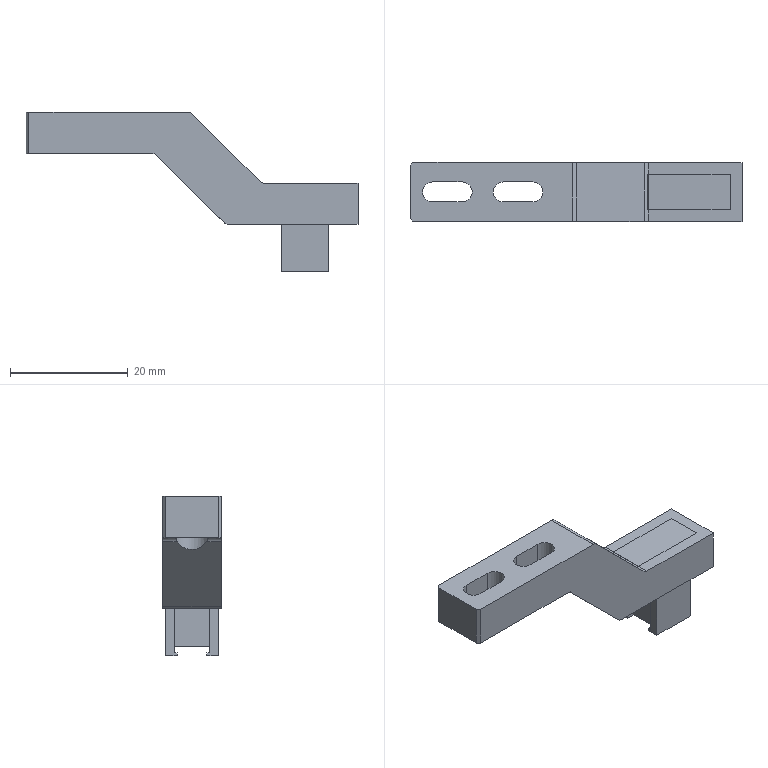NC program | NX | posted with a generic post | part box 56.3 x 10 x 27 mm
Lines 2463 to 3920 of 3920:
(ZLEVEL_PROFILE_COPY_1_COPY , TOOL : D4R0.2)
N4900 T05 M6
N4902 G54
N4904 G17 G0 G90 X3.577 Y-6.289 S9500 M3
N4906 G43 Z30. H5
N4908 Z-6.511
N4910 G94 G1 Z-8.011 F800.
N4912 X4.098 Y-5.88
N4914 G3 X4.247 Y-5.509 R0.4
N4916 G1 X4.175 Y-5. F2000.
N4918 Y5.
N4920 X4.242 Y5.476
N4922 X4.254 Y5.53
N4924 X4.194 Y5.54 Z-8.023
N4926 X4.108 Y5.
N4928 Y-5.
N4930 X4.186 Y-5.505
N4932 X4.154 Y-5.504 Z-8.029
N4934 X4.079 Y-5.
N4936 Y5.
N4938 G2 X4.166 Y5.547 R2.006
N4940 G1 X4.13 Y5.551 Z-8.038
N4942 X4.095 Y5.555 Z-8.047
N4944 X4.008 Y5.
N4946 Y-5.
N4948 X4.08 Y-5.501
N4950 X4.037 Y-5.503 Z-8.061
N4952 X3.994 Y-5.505 Z-8.074
N4954 X3.924 Y-5.
N4956 Y5.
N4958 X3.988 Y5.476
N4960 X4.009 Y5.55
N4962 X3.923 Y5.537 Z-8.109
N4964 X3.84 Y5.
N4966 Y-5.
N4968 X3.913 Y-5.503
N4970 X3.865 Y-5.502 Z-8.13
N4972 X3.825 Y-5.5 Z-8.15
N4974 X3.758 Y-5.
N4976 Y5.
N4978 X3.83 Y5.518
N4980 X3.791 Y5.517 Z-8.175
N4982 X3.749 Y5.516 Z-8.199
N4984 X3.678 Y5.
N4986 Y-5.
N4988 X3.747 Y-5.502
N4990 X3.708 Z-8.227
N4992 X3.667 Z-8.255
N4994 X3.6 Y-5.
N4996 Y5.
N4998 X3.668 Y5.511
N5000 X3.631 Y5.507 Z-8.286
N5002 X3.588 Y5.503 Z-8.317
N5004 G3 X3.527 Y5. R5.351
N5006 G1 Y-5.
N5008 G3 X3.589 Y-5.501 R2.547
N5010 G1 X3.549 Y-5.5 Z-8.35
N5012 X3.513 Z-8.384
N5014 G2 X3.458 Y-5. R31.618
N5016 G1 Y5.
N5018 X3.511 Y5.5
N5020 X3.47 Z-8.418
N5022 X3.439 Z-8.452
N5024 X3.39 Y5.
N5026 Y-5.
N5028 G3 X3.441 Y-5.5 R21.316
N5030 G1 X3.404 Z-8.487
N5032 X3.369 Z-8.521
N5034 G2 X3.32 Y-5. R27.436
N5036 G1 Y5.
N5038 X3.366 Y5.5
N5040 X3.326 Z-8.556
N5042 X3.292 Z-8.591
N5044 X3.25 Y5.
N5046 Y-5.
N5048 G3 X3.295 Y-5.5 R22.467
N5050 G1 X3.258 Z-8.626
N5052 X3.222 Z-8.662
N5054 G2 X3.179 Y-5. R2.843
N5056 G1 Y5.
N5058 X3.218 Y5.5
N5060 X3.18 Z-8.697
N5062 X3.145 Z-8.732
N5064 X3.108 Y5.
N5066 Y-5.
N5068 G3 X3.148 Y-5.5 R26.717
N5070 G1 X3.111 Z-8.767
N5072 X3.075 Z-8.803
N5074 X3.037 Y-5.
N5076 Y5.
N5078 X3.072 Y5.5
N5080 X3.034 Z-8.838
N5082 X2.999 Z-8.873
N5084 X2.966 Y5.
N5086 Y-5.
N5088 X3.001 Y-5.5
N5090 X2.964 Z-8.908
N5092 X2.928 Z-8.944
N5094 X2.895 Y-5.
N5096 Y5.
N5098 X2.926 Y5.5
N5100 X2.888 Z-8.979
N5102 X2.853 Z-9.014
N5104 X2.825 Y5.
N5106 Y-5.
N5108 X2.854 Y-5.5
N5110 X2.817 Z-9.05
N5112 X2.781 Z-9.085
N5114 X2.754 Y-5.
N5116 Y5.
N5118 X2.779 Y5.5
N5120 X2.741 Z-9.12
N5122 X2.706 Z-9.155
N5124 X2.683 Y5.
N5126 Y-5.
N5128 X2.707 Y-5.5
N5130 X2.67 Z-9.191
N5132 X2.635 Z-9.226
N5134 X2.612 Y-5.
N5136 Y5.
N5138 X2.633 Y5.5
N5140 X2.595 Z-9.261
N5142 X2.56 Z-9.296
N5144 X2.541 Y5.
N5146 Y-5.
N5148 X2.561 Y-5.5
N5150 X2.524 Z-9.332
N5152 X2.488 Z-9.367
N5154 X2.47 Y-5.
N5156 Y5.
N5158 X2.487 Y5.5
N5160 X2.449 Z-9.402
N5162 X2.414 Z-9.437
N5164 X2.399 Y5.
N5166 Y-5.
N5168 X2.415 Y-5.5
N5170 X2.378 Z-9.473
N5172 X2.342 Z-9.508
N5174 X2.328 Y-5.
N5176 Y5.
N5178 X2.34 Y5.5
N5180 X2.302 Z-9.543
N5182 X2.267 Z-9.578
N5184 X2.257 Y5.
N5186 Y-5.
N5188 X2.269 Y-5.5
N5190 X2.232 Z-9.614
N5192 X2.196 Z-9.649
N5194 X2.195 Y-5.476
N5196 X2.186 Y-5.
N5198 Y5.
N5200 X2.194 Y5.5
N5202 X2.156 Z-9.684
N5204 X2.122 Z-9.719
N5206 X2.115 Y5.
N5208 Y-5.
N5210 X2.124 Y-5.5
N5212 X2.087 Z-9.755
N5214 X2.053 Z-9.79
N5216 X2.045 Y-5.
N5218 Y5.
N5220 X2.05 Y5.5
N5222 X2.012 Z-9.825
N5224 X1.979 Z-9.86
N5226 X1.974 Y5.
N5228 Y-5.
N5230 X1.981 Y-5.5
N5232 X1.944 Z-9.896
N5234 X1.91 Z-9.931
N5236 X1.903 Y-5.
N5238 Y5.
N5240 X1.907 Y5.5
N5242 X1.87 Z-9.966
N5244 X1.836 Z-10.001
N5246 X1.832 Y5.
N5248 Y-5.
N5250 X1.838 Y-5.5
N5252 X1.802 Z-10.037
N5254 X1.767 Z-10.072
N5256 X1.761 Y-5.
N5258 Y5.
N5260 X1.765 Y5.5
N5262 X1.728 Z-10.107
N5264 X1.694 Z-10.142
N5266 X1.69 Y5.
N5268 Y-5.
N5270 X1.696 Y-5.5
N5272 X1.659 Z-10.178
N5274 X1.625 Z-10.213
N5276 X1.619 Y-5.
N5278 Y5.
N5280 X1.623 Y5.5
N5282 X1.586 Z-10.248
N5284 X1.552 Z-10.283
N5286 X1.548 Y5.
N5288 Y-5.
N5290 X1.553 Y-5.5
N5292 X1.517 Z-10.319
N5294 X1.482 Z-10.354
N5296 X1.477 Y-5.
N5298 Y5.
N5300 X1.481 Y5.5
N5302 X1.444 Z-10.389
N5304 X1.41 Z-10.424
N5306 X1.406 Y5.
N5308 Y-5.
N5310 X1.409 Y-5.476
N5312 X1.411 Y-5.5
N5314 X1.374 Z-10.46
N5316 X1.34 Z-10.495
N5318 X1.338 Y-5.476
N5320 X1.335 Y-5.
N5322 Y5.
N5324 X1.337 Y5.476
N5326 X1.339 Y5.5
N5328 X1.302 Z-10.53
N5330 X1.268 Z-10.565
N5332 X1.266 Y5.476
N5334 X1.265 Y5.
N5336 Y-5.
N5338 X1.267 Y-5.476
N5340 X1.268 Y-5.5
N5342 X1.232 Z-10.601
N5344 X1.197 Z-10.636
N5346 X1.196 Y-5.476
N5348 X1.194 Y-5.
N5350 Y5.
N5352 X1.195 Y5.476
N5354 X1.196 Y5.5
N5356 X1.159 Z-10.671
N5358 X1.125 Z-10.707
N5360 X1.124 Y5.476
N5362 X1.123 Y5.
N5364 Y-5.
N5366 X1.124 Y-5.476
N5368 X1.126 Y-5.5
N5370 X1.089 Z-10.742
N5372 X1.055 Z-10.777
N5374 X1.053 Y-5.476
N5376 X1.052 Y-5.
N5378 Y5.
N5380 X1.053 Y5.476
N5382 X1.054 Y5.5
N5384 X1.017 Z-10.812
N5386 X0.983 Z-10.848
N5388 X0.982 Y5.476
N5390 X0.981 Y5.
N5392 Y-5.
N5394 X0.982 Y-5.476
N5396 X0.984 Y-5.5
N5398 X0.947 Z-10.883
N5400 X0.912 Z-10.918
N5402 X0.911 Y-5.476
N5404 X0.91 Y-5.
N5406 Y5.
N5408 X0.911 Y5.476
N5410 X0.912 Y5.5
N5412 X0.875 Z-10.953
N5414 X0.841 Z-10.989
N5416 X0.84 Y5.476
N5418 X0.839 Y5.
N5420 Y-5.
N5422 X0.84 Y-5.476
N5424 X0.841 Y-5.5
N5426 X0.804 Z-11.024
N5428 X0.77 Z-11.059
N5430 X0.769 Y-5.476
N5432 X0.768 Y-5.
N5434 Y5.
N5436 X0.769 Y5.476
N5438 X0.77 Y5.5
N5440 X0.733 Z-11.094
N5442 X0.699 Z-11.13
N5444 X0.698 Y5.476
N5446 X0.697 Y5.
N5448 Y-5.
N5450 X0.698 Y-5.476
N5452 X0.699 Y-5.5
N5454 X0.662 Z-11.165
N5456 X0.628 Z-11.2
N5458 X0.627 Y-5.476
N5460 X0.626 Y-5.
N5462 Y5.
N5464 X0.627 Y5.476
N5466 X0.628 Y5.5
N5468 X0.591 Z-11.235
N5470 X0.557 Z-11.271
N5472 X0.556 Y5.476
N5474 X0.555 Y5.
N5476 Y-5.
N5478 X0.556 Y-5.476
N5480 X0.557 Y-5.5
N5482 X0.52 Z-11.306
N5484 X0.486 Z-11.341
N5486 X0.485 Y-5.476
N5488 Y-5.
N5490 Y5.
N5492 Y5.476
N5494 X0.486 Y5.5
N5496 X0.449 Z-11.376
N5498 X0.415 Z-11.412
N5500 X0.414 Y5.476
N5502 Y5.
N5504 Y-5.
N5506 Y-5.476
N5508 X0.415 Y-5.5
N5510 X0.379 Z-11.447
N5512 X0.344 Z-11.482
N5514 X0.343 Y-5.476
N5516 Y-5.
N5518 Y5.
N5520 Y5.476
N5522 X0.344 Y5.5
N5524 X0.307 Z-11.517
N5526 X0.273 Z-11.553
N5528 X0.272 Y5.476
N5530 Y5.
N5532 Y-5.
N5534 Y-5.476
N5536 X0.274 Y-5.5
N5538 X0.237 Z-11.588
N5540 X0.203 Z-11.623
N5542 X0.201 Y-5.476
N5544 Y-5.
N5546 Y5.
N5548 Y5.476
N5550 X0.202 Y5.5
N5552 X0.166 Z-11.658
N5554 X0.132 Z-11.694
N5556 X0.13 Y5.476
N5558 Y5.
N5560 Y-5.
N5562 Y-5.476
N5564 X0.132 Y-5.5
N5566 X0.095 Z-11.729
N5568 X0.061 Z-11.764
N5570 X0.059 Y-5.476
N5572 Y-5.
N5574 Y5.
N5576 Y5.476
N5578 X0.061 Y5.5
N5580 X0.024 Z-11.799
N5582 X-0.01 Z-11.835
N5584 X-0.012 Y5.476
N5586 Y5.
N5588 Y-5.
N5590 Y-5.476
N5592 X-0.01 Y-5.5
N5594 X-0.047 Z-11.87
N5596 X-0.081 Z-11.905
N5598 X-0.083 Y-5.476
N5600 Y-5.
N5602 Y5.
N5604 Y5.476
N5606 X-0.081 Y5.5
N5608 X-0.118 Z-11.94
N5610 X-0.152 Z-11.976
N5612 X-0.154 Y5.476
N5614 Y5.
N5616 Y-5.
N5618 X-0.153 Y-5.476
N5620 X-0.152 Y-5.5
N5622 X-0.189 Z-12.011
N5624 X-0.223 Z-12.046
N5626 X-0.224 Y-5.476
N5628 X-0.225 Y-5.
N5630 Y5.
N5632 X-0.224 Y5.476
N5634 X-0.223 Y5.5
N5636 X-0.26 Z-12.081
N5638 X-0.294 Z-12.117
N5640 X-0.295 Y5.476
N5642 Y5.
N5644 Y-5.
N5646 Y-5.476
N5648 X-0.294 Y-5.5
N5650 X-0.331 Z-12.152
N5652 X-0.365 Z-12.187
N5654 X-0.366 Y-5.476
N5656 Y-5.
N5658 Y5.
N5660 Y5.476
N5662 X-0.365 Y5.5
N5664 X-0.402 Z-12.222
N5666 X-0.436 Z-12.258
N5668 X-0.437 Y5.476
N5670 Y5.
N5672 Y-5.
N5674 Y-5.476
N5676 X-0.436 Y-5.5
N5678 X-0.473 Z-12.293
N5680 X-0.507 Z-12.328
N5682 X-0.508 Y-5.476
N5684 Y-5.
N5686 Y5.
N5688 Y5.476
N5690 X-0.507 Y5.5
N5692 X-0.544 Z-12.364
N5694 X-0.578 Z-12.399
N5696 X-0.579 Y5.476
N5698 Y5.
N5700 Y-5.
N5702 Y-5.476
N5704 X-0.578 Y-5.5
N5706 X-0.615 Z-12.434
N5708 X-0.649 Z-12.469
N5710 X-0.65 Y-5.476
N5712 Y-5.
N5714 Y5.
N5716 Y5.476
N5718 X-0.649 Y5.5
N5720 X-0.685 Z-12.505
N5722 X-0.719 Z-12.54
N5724 X-0.721 Y5.476
N5726 Y5.
N5728 Y-5.
N5730 Y-5.476
N5732 X-0.719 Y-5.5
N5734 X-0.756 Z-12.575
N5736 X-0.79 Z-12.61
N5738 X-0.792 Y-5.476
N5740 Y-5.
N5742 Y5.
N5744 Y5.476
N5746 X-0.79 Y5.5
N5748 X-0.827 Z-12.646
N5750 X-0.861 Z-12.681
N5752 X-0.863 Y5.476
N5754 Y5.
N5756 Y-5.
N5758 Y-5.476
N5760 X-0.861 Y-5.5
N5762 X-0.898 Z-12.716
N5764 X-0.932 Z-12.751
N5766 X-0.934 Y-5.476
N5768 Y-5.
N5770 Y5.
N5772 Y5.476
N5774 X-0.932 Y5.5
N5776 X-0.969 Z-12.787
N5778 X-1.003 Z-12.822
N5780 X-1.005 Y5.476
N5782 Y5.
N5784 Y-5.
N5786 Y-5.476
N5788 X-1.003 Y-5.5
N5790 X-1.04 Z-12.857
N5792 X-1.074 Z-12.892
N5794 X-1.075 Y-5.476
N5796 Y-5.
N5798 Y5.
N5800 Y5.476
N5802 X-1.074 Y5.5
N5804 X-1.111 Z-12.928
N5806 X-1.145 Z-12.963
N5808 X-1.146 Y5.476
N5810 Y5.
N5812 Y-5.
N5814 Y-5.476
N5816 X-1.145 Y-5.5
N5818 X-1.182 Z-12.998
N5820 X-1.216 Z-13.033
N5822 X-1.217 Y-5.476
N5824 Y-5.
N5826 Y5.
N5828 Y5.476
N5830 X-1.216 Y5.5
N5832 X-1.253 Z-13.069
N5834 X-1.287 Z-13.104
N5836 X-1.288 Y5.476
N5838 Y5.
N5840 Y-5.
N5842 Y-5.476
N5844 X-1.287 Y-5.5
N5846 X-1.324 Z-13.139
N5848 X-1.358 Z-13.174
N5850 X-1.359 Y-5.476
N5852 Y-5.
N5854 Y5.
N5856 Y5.476
N5858 X-1.358 Y5.5
N5860 X-1.395 Z-13.21
N5862 X-1.429 Z-13.245
N5864 X-1.43 Y5.476
N5866 Y5.
N5868 Y-5.
N5870 Y-5.476
N5872 X-1.429 Y-5.5
N5874 X-1.465 Z-13.28
N5876 X-1.499 Z-13.315
N5878 X-1.501 Y-5.476
N5880 Y-5.
N5882 Y5.
N5884 Y5.476
N5886 X-1.499 Y5.5
N5888 X-1.536 Z-13.351
N5890 X-1.57 Z-13.386
N5892 X-1.572 Y5.476
N5894 Y5.
N5896 Y-5.
N5898 Y-5.476
N5900 X-1.57 Y-5.5
N5902 X-1.607 Z-13.421
N5904 X-1.641 Z-13.456
N5906 X-1.643 Y-5.476
N5908 Y-5.
N5910 Y5.
N5912 Y5.476
N5914 X-1.641 Y5.5
N5916 X-1.678 Z-13.492
N5918 X-1.712 Z-13.527
N5920 X-1.714 Y5.476
N5922 Y5.
N5924 Y-5.
N5926 Y-5.476
N5928 X-1.712 Y-5.5
N5930 X-1.749 Z-13.562
N5932 X-1.784 Z-13.597
N5934 X-1.785 Y-5.
N5936 Y5.
N5938 X-1.784 Y5.5
N5940 X-1.82 Z-13.633
N5942 X-1.854 Z-13.668
N5944 X-1.855 Y5.476
N5946 Y5.
N5948 Y-5.
N5950 Y-5.476
N5952 X-1.854 Y-5.5
N5954 X-1.891 Z-13.703
N5956 X-1.925 Z-13.738
N5958 X-1.926 Y-5.476
N5960 Y-5.
N5962 Y5.
N5964 Y5.476
N5966 X-1.925 Y5.5
N5968 X-1.962 Z-13.774
N5970 X-1.996 Z-13.809
N5972 X-1.997 Y5.476
N5974 Y5.
N5976 Y-5.
N5978 Y-5.476
N5980 X-1.996 Y-5.5
N5982 X-2.033 Z-13.844
N5984 X-2.067 Z-13.88
N5986 X-2.068 Y-5.
N5988 Y5.
N5990 X-2.067 Y5.5
N5992 X-2.104 Z-13.915
N5994 X-2.138 Z-13.95
N5996 X-2.139 Y5.476
N5998 Y5.
N6000 Y-5.
N6002 Y-5.476
N6004 X-2.138 Y-5.5
N6006 X-2.175 Z-13.985
N6008 X-2.209 Z-14.021
N6010 X-2.21 Y-5.476
N6012 Y-5.
N6014 Y5.
N6016 Y5.476
N6018 X-2.209 Y5.5
N6020 X-2.245 Z-14.056
N6022 X-2.28 Z-14.091
N6024 X-2.281 Y5.476
N6026 Y5.
N6028 Y-5.
N6030 Y-5.476
N6032 X-2.28 Y-5.5
N6034 X-2.316 Z-14.126
N6036 X-2.351 Z-14.162
N6038 X-2.352 Y-5.
N6040 Y5.
N6042 X-2.351 Y5.5
N6044 X-2.387 Z-14.197
N6046 X-2.421 Z-14.232
N6048 X-2.423 Y5.476
N6050 Y5.
N6052 Y-5.
N6054 Y-5.476
N6056 X-2.421 Y-5.5
N6058 X-2.458 Z-14.267
N6060 X-2.492 Z-14.303
N6062 X-2.494 Y-5.476
N6064 Y-5.
N6066 Y5.
N6068 Y5.476
N6070 X-2.492 Y5.5
N6072 X-2.529 Z-14.338
N6074 X-2.563 Z-14.373
N6076 X-2.565 Y5.476
N6078 Y5.
N6080 Y-5.
N6082 Y-5.476
N6084 X-2.563 Y-5.5
N6086 X-2.6 Z-14.408
N6088 X-2.634 Z-14.444
N6090 X-2.635 Y-5.476
N6092 Y-5.
N6094 Y5.
N6096 Y5.476
N6098 X-2.634 Y5.5
N6100 X-2.671 Z-14.479
N6102 X-2.705 Z-14.514
N6104 X-2.706 Y5.476
N6106 Y5.
N6108 Y-5.
N6110 Y-5.476
N6112 X-2.705 Y-5.5
N6114 X-2.742 Z-14.549
N6116 X-2.776 Z-14.585
N6118 X-2.777 Y-5.476
N6120 Y-5.
N6122 Y5.
N6124 Y5.476
N6126 X-2.776 Y5.5
N6128 X-2.813 Z-14.62
N6130 X-2.847 Z-14.655
N6132 X-2.848 Y5.476
N6134 Y5.
N6136 Y-5.
N6138 Y-5.476
N6140 X-2.847 Y-5.5
N6142 X-2.884 Z-14.69
N6144 X-2.918 Z-14.726
N6146 X-2.919 Y-5.476
N6148 Y-5.
N6150 Y5.
N6152 Y5.476
N6154 X-2.918 Y5.5
N6156 X-2.955 Z-14.761
N6158 X-2.989 Z-14.796
N6160 X-2.99 Y5.476
N6162 Y5.
N6164 Y-5.
N6166 Y-5.476
N6168 X-2.989 Y-5.5
N6170 X-3.025 Z-14.831
N6172 X-3.06 Z-14.867
N6174 X-3.061 Y-5.476
N6176 Y-5.
N6178 Y5.
N6180 Y5.476
N6182 X-3.06 Y5.5
N6184 X-3.096 Z-14.902
N6186 X-3.13 Z-14.937
N6188 X-3.132 Y5.476
N6190 Y5.
N6192 Y-5.
N6194 Y-5.476
N6196 X-3.13 Y-5.5
N6198 X-3.167 Z-14.972
N6200 X-3.201 Z-15.008
N6202 X-3.203 Y-5.476
N6204 Y-5.
N6206 Y5.
N6208 Y5.476
N6210 X-3.201 Y5.5
N6212 X-3.238 Z-15.043
N6214 X-3.272 Z-15.078
N6216 X-3.274 Y5.476
N6218 Y5.
N6220 Y-5.
N6222 Y-5.476
N6224 X-3.272 Y-5.5
N6226 X-3.309 Z-15.113
N6228 X-3.343 Z-15.149
N6230 X-3.345 Y-5.476
N6232 Y-5.
N6234 Y5.
N6236 Y5.476
N6238 X-3.343 Y5.5
N6240 X-3.38 Z-15.184
N6242 X-3.414 Z-15.219
N6244 X-3.416 Y5.476
N6246 X-3.415 Y5.
N6248 Y-5.
N6250 Y-5.476
N6252 X-3.414 Y-5.5
N6254 X-3.451 Z-15.254
N6256 X-3.485 Z-15.29
N6258 X-3.486 Y-5.476
N6260 Y-5.
N6262 Y5.
N6264 Y5.476
N6266 X-3.485 Y5.5
N6268 X-3.522 Z-15.325
N6270 X-3.556 Z-15.36
N6272 X-3.557 Y5.476
N6274 Y5.
N6276 Y-5.
N6278 Y-5.476
N6280 X-3.556 Y-5.5
N6282 X-3.593 Z-15.395
N6284 X-3.627 Z-15.431
N6286 X-3.628 Y-5.476
N6288 Y-5.
N6290 Y5.
N6292 Y5.476
N6294 X-3.627 Y5.5
N6296 X-3.664 Z-15.466
N6298 X-3.698 Z-15.501
N6300 X-3.699 Y5.476
N6302 Y5.
N6304 Y-5.
N6306 Y-5.476
N6308 X-3.698 Y-5.5
N6310 X-3.735 Z-15.537
N6312 X-3.769 Z-15.572
N6314 X-3.77 Y-5.476
N6316 Y-5.
N6318 Y5.
N6320 Y5.476
N6322 X-3.769 Y5.5
N6324 X-3.806 Z-15.607
N6326 X-3.84 Z-15.642
N6328 X-3.841 Y5.476
N6330 Y5.
N6332 Y-5.
N6334 Y-5.476
N6336 X-3.84 Y-5.5
N6338 X-3.876 Z-15.678
N6340 X-3.91 Z-15.713
N6342 X-3.912 Y-5.476
N6344 Y-5.
N6346 Y5.
N6348 Y5.476
N6350 X-3.911 Y5.5
N6352 X-3.947 Z-15.748
N6354 X-3.981 Z-15.783
N6356 X-3.983 Y5.476
N6358 Y5.
N6360 Y-5.
N6362 Y-5.476
N6364 X-3.981 Y-5.5
N6366 X-4.018 Z-15.819
N6368 X-4.052 Z-15.854
N6370 X-4.054 Y-5.476
N6372 Y-5.
N6374 Y5.
N6376 Y5.476
N6378 X-4.052 Y5.5
N6380 X-4.089 Z-15.889
N6382 X-4.123 Z-15.924
N6384 X-4.125 Y5.476
N6386 Y5.
N6388 Y-5.
N6390 Y-5.476
N6392 X-4.123 Y-5.5
N6394 X-4.16 Z-15.96
N6396 X-4.194 Z-15.995
N6398 X-4.196 Y-5.476
N6400 X-4.195 Y-5.
N6402 Y5.
N6404 X-4.196 Y5.476
N6406 X-4.194 Y5.5
N6408 X-4.231 Z-16.03
N6410 X-4.265 Z-16.065
N6412 X-4.267 Y5.476
N6414 X-4.266 Y5.
N6416 Y-5.
N6418 X-4.267 Y-5.476
N6420 X-4.265 Y-5.5
N6422 X-4.302 Z-16.101
N6424 X-4.336 Z-16.136
N6426 X-4.337 Y-5.476
N6428 Y-5.
N6430 Y5.
N6432 X-4.338 Y5.476
N6434 X-4.336 Y5.5
N6436 X-4.373 Z-16.171
N6438 X-4.407 Z-16.206
N6440 X-4.408 Y5.476
N6442 Y5.
N6444 Y-5.
N6446 Y-5.476
N6448 X-4.407 Y-5.5
N6450 X-4.444 Z-16.242
N6452 X-4.478 Z-16.277
N6454 X-4.479 Y-5.476
N6456 Y-5.
N6458 Y5.
N6460 Y5.476
N6462 X-4.478 Y5.5
N6464 X-4.515 Z-16.312
N6466 X-4.549 Z-16.347
N6468 X-4.55 Y5.476
N6470 Y5.
N6472 Y-5.
N6474 Y-5.476
N6476 X-4.549 Y-5.5
N6478 X-4.586 Z-16.383
N6480 X-4.62 Z-16.418
N6482 X-4.621 Y-5.476
N6484 Y-5.
N6486 Y5.
N6488 Y5.476
N6490 X-4.62 Y5.5
N6492 X-4.657 Z-16.453
N6494 X-4.691 Z-16.488
N6496 X-4.692 Y5.476
N6498 Y5.
N6500 Y-5.
N6502 Y-5.476
N6504 X-4.691 Y-5.5
N6506 X-4.727 Z-16.524
N6508 X-4.762 Z-16.559
N6510 X-4.763 Y-5.476
N6512 Y-5.
N6514 Y5.
N6516 Y5.476
N6518 X-4.762 Y5.5
N6520 X-4.799 Z-16.594
N6522 X-4.833 Z-16.629
N6524 X-4.834 Y5.476
N6526 Y5.
N6528 Y-5.
N6530 Y-5.476
N6532 X-4.832 Y-5.5
N6534 X-4.869 Z-16.665
N6536 X-4.903 Z-16.7
N6538 X-4.905 Y-5.476
N6540 Y-5.
N6542 Y5.
N6544 Y5.476
N6546 X-4.904 Y5.5
N6548 X-4.941 Z-16.735
N6550 X-4.975 Z-16.77
N6552 X-4.976 Y5.476
N6554 Y5.
N6556 Y-5.
N6558 Y-5.476
N6560 X-4.975 Y-5.5
N6562 X-5.011 Z-16.806
N6564 X-5.046 Z-16.841
N6566 X-5.047 Y-5.476
N6568 X-5.046 Y-5.
N6570 Y5.
N6572 X-5.047 Y5.476
N6574 X-5.046 Y5.5
N6576 X-5.083 Z-16.876
N6578 X-5.117 Z-16.911
N6580 X-5.119 Y5.476
N6582 X-5.117 Y5.
N6584 Y-5.
N6586 X-5.118 Y-5.476
N6588 X-5.117 Y-5.5
N6590 X-5.154 Z-16.947
N6592 X-5.188 Z-16.982
N6594 X-5.189 Y-5.476
N6596 X-5.188 Y-5.
N6598 Y5.
N6600 X-5.19 Y5.476
N6602 X-5.188 Y5.5
N6604 X-5.225 Z-17.017
N6606 X-5.26 Z-17.053
N6608 X-5.261 Y5.476
N6610 X-5.259 Y5.
N6612 Y-5.
N6614 X-5.26 Y-5.476
N6616 X-5.259 Y-5.5
N6618 X-5.296 Z-17.088
N6620 X-5.33 Z-17.123
N6622 X-5.331 Y-5.476
N6624 X-5.33 Y-5.
N6626 Y5.
N6628 X-5.332 Y5.476
N6630 X-5.331 Y5.5
N6632 X-5.368 Z-17.158
N6634 X-5.402 Z-17.194
N6636 X-5.403 Y5.476
N6638 X-5.401 Y5.
N6640 Y-5.
N6642 X-5.402 Y-5.476
N6644 X-5.401 Y-5.5
N6646 X-5.438 Z-17.229
N6648 X-5.472 Z-17.264
N6650 X-5.473 Y-5.476
N6652 X-5.472 Y-5.
N6654 Y5.
N6656 X-5.474 Y5.476
N6658 X-5.473 Y5.5
N6660 X-5.51 Z-17.299
N6662 X-5.544 Z-17.335
N6664 X-5.546 Y5.476
N6666 X-5.543 Y5.
N6668 Y-5.
N6670 X-5.544 Y-5.476
N6672 X-5.543 Y-5.5
N6674 X-5.58 Z-17.37
N6676 X-5.614 Z-17.405
N6678 X-5.615 Y-5.476
N6680 X-5.614 Y-5.
N6682 Y5.
N6684 X-5.617 Y5.476
N6686 X-5.615 Y5.5
N6688 X-5.653 Z-17.44
N6690 X-5.687 Z-17.476
N6692 X-5.688 Y5.476
N6694 X-5.685 Y5.
N6696 Y-5.
N6698 Y-5.5
N6700 X-5.722 Z-17.511
N6702 X-5.756 Z-17.546
N6704 Y-5.
N6706 Y5.
N6708 X-5.759 Y5.476
N6710 X-5.758 Y5.5
N6712 X-5.795 Z-17.581
N6714 X-5.829 Z-17.617
N6716 X-5.83 Y5.476
N6718 X-5.826 Y5.
N6720 Y-5.
N6722 X-5.827 Y-5.5
N6724 X-5.864 Z-17.652
N6726 X-5.898 Z-17.687
N6728 X-5.897 Y-5.
N6730 Y5.
N6732 X-5.902 Y5.476
N6734 X-5.9 Y5.5
N6736 X-5.937 Z-17.722
N6738 X-5.971 Z-17.758
N6740 X-5.973 Y5.476
N6742 X-5.968 Y5.
N6744 Y-5.
N6746 X-5.969 Y-5.5
N6748 X-6.006 Z-17.793
N6750 X-6.041 Z-17.828
N6752 X-6.039 Y-5.
N6754 Y5.
N6756 X-6.044 Y5.476
N6758 X-6.043 Y5.5
N6760 X-6.08 Z-17.863
N6762 X-6.114 Z-17.899
N6764 X-6.116 Y5.476
N6766 X-6.11 Y5.
N6768 Y-5.
N6770 X-6.113 Y-5.476
N6772 X-6.112 Y-5.5
N6774 X-6.148 Z-17.934
N6776 X-6.183 Z-17.969
N6778 X-6.185 Y-5.476
N6780 X-6.181 Y-5.
N6782 Y5.
N6784 X-6.187 Y5.476
N6786 X-6.186 Y5.5
N6788 X-6.223 Z-18.004
N6790 X-6.257 Z-18.04
N6792 X-6.258 Y5.476
N6794 X-6.252 Y5.
N6796 Y-5.
N6798 X-6.256 Y-5.476
N6800 X-6.255 Y-5.5
N6802 X-6.292 Z-18.075
N6804 X-6.327 Z-18.11
N6806 X-6.323 Y-5.
N6808 Y5.
N6810 X-6.331 Y5.476
N6812 X-6.33 Y5.5
N6814 X-6.368 Z-18.145
N6816 X-6.403 Z-18.181
N6818 X-6.405 Y5.476
N6820 X-6.394 Y5.
N6822 Y-5.
N6824 X-6.4 Y-5.5
N6826 X-6.438 Z-18.216
N6828 X-6.473 Z-18.251
N6830 X-6.474 Y-5.476
N6832 X-6.465 Y-5.
N6834 Y5.
N6836 X-6.478 Y5.476
N6838 X-6.476 Y5.5
N6840 X-6.514 Z-18.286
N6842 X-6.549 Z-18.322
N6844 X-6.551 Y5.476
N6846 X-6.536 Y5.
N6848 Y-4.928
N6850 X-6.541 Y-4.94
N6852 X-6.545 Y-5.5
N6854 X-6.583 Z-18.357
N6856 X-6.618 Z-18.392
N6858 X-6.612 Y-4.925
N6860 X-6.606 Y-4.916
N6862 Y5.
N6864 X-6.623 Y5.5
N6866 X-6.661 Z-18.427
N6868 X-6.696 Z-18.463
N6870 X-6.677 Y5.
N6872 Y1.521
N6874 Y0.365
N6876 X-6.675 Y-0.352
N6878 X-6.677 Y-0.421
N6880 Y-4.896
N6882 X-6.683 Y-4.915
N6884 X-6.691 Y-5.5
N6886 X-6.729 Z-18.498
N6888 X-6.764 Z-18.533
N6890 X-6.765 Y-5.476
N6892 X-6.754 Y-4.909
N6894 X-6.748 Y-4.892
N6896 Y-0.702
N6898 X-6.747 Y-0.67
N6900 X-6.708 Y-0.14
N6902 G3 X-6.747 Y0.67 R8.918
N6904 G1 X-6.748 Y0.702
N6906 Y5.
N6908 X-6.77 Y5.476
N6910 X-6.769 Y5.5
N6912 X-6.807 Z-18.568
N6914 X-6.842 Z-18.604
N6916 X-6.819 Y5.
N6918 Y1.741
N6920 Y0.983
N6922 X-6.816 Y0.865
N6924 G3 X-6.751 Y0.287 R2.493
N6926 G2 X-6.751 Y-0.287 R1.264
N6928 G3 X-6.816 Y-0.865 R2.493
N6930 G1 X-6.819 Y-0.983
N6932 Y-1.741
N6934 Y-4.889
N6936 X-6.825 Y-4.905
N6938 X-6.837 Y-5.5
N6940 X-6.874 Z-18.639
N6942 X-6.909 Z-18.674
N6944 X-6.89 Y-4.887
N6946 Y-1.834
N6948 X-6.888 Y-1.019
N6950 G2 X-6.752 Y-0.211 R2.855
N6952 G3 X-6.752 Y0.203 R0.676
N6954 G2 X-6.888 Y1.019 R2.85
N6956 G1 X-6.89 Y1.834
N6958 Y5.
N6960 X-6.915 Y5.5
N6962 X-6.954 Z-18.71
N6964 X-6.989 Z-18.745
N6966 X-6.961 Y5.
N6968 Y1.924
N6970 Y1.264
N6972 X-6.957 Y1.146
N6974 G3 X-6.739 Y0.14 R2.705
N6976 G1 Y-0.14
N6978 G3 X-6.957 Y-1.146 R2.741
N6980 G1 X-6.961 Y-1.264
N6982 Y-1.924
N6984 Y-4.882
N6986 X-6.967 Y-4.897
N6988 X-6.982 Y-5.5
N6990 X-7.02 Z-18.78
N6992 X-7.055 Z-18.815
N6994 X-7.038 Y-4.892
N6996 X-7.032 Y-4.877
N6998 Y-2.004
N7000 Y-1.272
N7002 G2 X-6.836 Y-0.344 R2.572
N7004 G1 X-6.743 Y-0.14
N7006 Y0.14
N7008 X-6.836 Y0.345
N7010 G2 X-7.032 Y1.272 R2.513
N7012 G1 Y2.004
N7014 Y5.
N7016 X-7.062 Y5.5
N7018 X-7.1 Z-18.851
N7020 X-7.135 Z-18.886
N7022 X-7.136 Y5.476
N7024 X-7.109 Y4.996
N7026 X-7.103 Y4.986
N7028 Y2.081
N7030 X-7.101 Y1.375
N7032 G3 X-6.743 Y0.14 R2.477
N7034 G1 Y-0.14
N7036 G3 X-7.101 Y-1.375 R2.477
N7038 G1 X-7.103 Y-2.081
N7040 Y-4.872
N7042 X-7.108 Y-4.887
N7044 X-7.128 Y-5.5
N7046 G2 X-7.339 Y-5.84 R0.4
N7048 G1 X-7.858 Y-6.118
N7050 Z-17.386
N7052 G0 Z30.
N7054 X-7.883 Y0.767
N7056 Z-17.456
N7058 G1 Z-18.956 F800.
N7060 X-7.352 Y1.111
N7062 G3 X-7.17 Y1.467 R0.4
N7064 G1 X-7.174 Y1.545 F2000.
N7066 Y2.152
N7068 Y4.969
N7070 X-7.18 Y4.985
N7072 X-7.21 Y5.476
N7074 X-7.208 Y5.5
N7076 X-7.246 Z-18.992
N7078 X-7.281 Z-19.027
N7080 X-7.283 Y5.476
N7082 X-7.25 Y4.972
N7084 X-7.245 Y4.956
N7086 Y2.218
N7088 X-7.244 Y1.554
N7090 X-7.313 Y1.631 Z-19.097
N7092 X-7.316 Y2.283
N7094 Y4.944
N7096 X-7.321 Y4.96
N7098 X-7.356 Y5.476
N7100 X-7.355 Y5.5
N7102 X-7.393 Y5.498 Z-19.133
N7104 X-7.428 Y5.497 Z-19.168
N7106 X-7.397 Y4.982
N7108 X-7.386 Y4.932
N7110 Y2.339
N7112 X-7.387 Y1.825
N7114 X-7.384 Y1.709
N7116 X-7.456 Y1.78 Z-19.238
N7118 X-7.458 Y1.825
N7120 X-7.457 Y2.395
N7122 Y4.925
N7124 X-7.463 Y4.935
N7126 X-7.502 Y5.49
N7128 X-7.539 Y5.487 Z-19.274
N7130 X-7.575 Y5.484 Z-19.309
N7132 G3 X-7.528 Y4.915 R8.475
N7134 G1 Y2.448
N7136 X-7.53 Y1.84
N7138 X-7.603 Y1.879 Z-19.379
N7140 Y2.387
N7142 X-7.599 Y2.497
N7144 Y4.9
N7146 X-7.605 Y4.915
N7148 X-7.649 Y5.477
N7150 X-7.681 Y5.483 Z-19.418
N7152 X-7.704 Y5.486 Z-19.457
N7154 G3 X-7.66 Y4.895 R4.03
N7156 G1 Y2.524
N7158 X-7.662 Y1.922
N7160 X-7.708 Y1.976 Z-19.54
N7162 G2 X-7.694 Y2.568 R4.379
N7164 G1 Y4.843
N7166 G2 X-7.747 Y5.497 R2.665
N7168 G1 X-7.767 Y5.498 Z-19.58
N7170 X-7.793 Y5.499 Z-19.62
N7172 G3 X-7.738 Y4.837 R2.098
N7174 G1 Y2.599
N7176 G3 X-7.753 Y2.031 R3.987
N7178 G1 X-7.816 Y2.084 Z-19.699
N7180 X-7.817 Y2.106
N7182 X-7.793 Y2.638
N7184 Y4.783
N7186 G2 X-7.855 Y5.495 R2.569
N7188 G1 X-7.885 Y5.497 Z-19.733
N7190 X-7.924 Y5.499 Z-19.768
N7192 G3 X-7.856 Y4.769 R2.537
N7194 G1 Y2.689
N7196 X-7.861 Y2.676
N7198 X-7.885 Y2.132
N7200 X-7.951 Y2.173 Z-19.828
N7202 X-7.936 Y2.668
N7204 X-7.923 Y2.731
N7206 Y4.738
N7208 G2 X-8.005 Y5.499 R2.222
N7210 G1 X-8.038 Z-19.853
N7212 X-8.081 Z-19.877
N7214 G3 X-7.993 Y4.719 R2.028
N7216 G1 Y2.768
N7218 X-8.017 Y2.668
N7220 X-8.03 Y2.224
N7222 X-8.096 Y2.266 Z-19.915
N7224 X-8.06 Y2.826
N7226 Y4.683
N7228 X-8.086 Y4.736
N7230 X-8.156 Y5.476
N7232 X-8.155 Y5.499
N7234 X-8.186 Z-19.929
N7236 X-8.214 Y5.5 Z-19.943
N7238 X-8.215 Y5.476
N7240 X-8.155 Y4.736
N7242 X-8.121 Y4.671
N7244 Y2.879
N7246 X-8.174 Y2.296
N7248 X-8.23 Y2.316 Z-19.962
N7250 X-8.174 Y2.924
N7252 Y4.72
N7254 G2 X-8.266 Y5.495 R1.95
N7256 G1 X-8.283 Y5.492 Z-19.968
N7258 X-8.318 Y5.486 Z-19.975
N7260 G3 X-8.222 Y4.72 R1.566
N7262 G1 Y2.949
N7264 X-8.258 Y2.873
N7266 X-8.293 Y2.387
N7268 X-8.292 Y2.363
N7270 X-8.312 Y2.477 Z-19.98
N7272 X-8.333 Y2.59 Z-19.985
N7274 X-8.264 Y2.964
N7276 Y4.744
N7278 G2 X-8.353 Y5.48 R1.36
N7280 G1 X-8.375 Y5.368 Z-19.988
N7282 X-8.389 Y5.254 Z-19.991
N7284 X-8.399 Y5.139 Z-19.994
N7286 X-8.417 Y5.023 Z-19.997
N7288 X-8.396 Y4.914 Z-20.
N7290 X-8.356 Y4.76
N7292 Y2.909
N7294 Z-18.5
N7296 G0 Z30.
N7298 X-7.909 Y-6.208
N7300 Z-17.456
N7302 G1 Z-18.956 F800.
N7304 X-7.379 Y-5.858
N7306 G3 X-7.201 Y-5.5 R0.4
N7308 G1 X-7.202 Y-5.476 F2000.
N7310 X-7.179 Y-4.887
N7312 X-7.174 Y-4.871
N7314 Y-2.152
N7316 Y-1.545
N7318 X-7.17 Y-1.467
N7320 X-7.244 Y-1.554 Z-19.027
N7322 X-7.245 Y-2.218
N7324 Y-4.871
N7326 X-7.25 Y-4.887
N7328 X-7.275 Y-5.476
N7330 X-7.274 Y-5.5
N7332 X-7.311 Z-19.062
N7334 X-7.346 Z-19.097
N7336 X-7.348 Y-5.476
N7338 X-7.325 Y-4.915
N7340 X-7.316 Y-4.871
N7342 Y-2.283
N7344 X-7.313 Y-1.631
N7346 X-7.384 Y-1.709 Z-19.168
N7348 X-7.387 Y-1.825
N7350 X-7.386 Y-2.339
N7352 Y-4.871
N7354 G3 X-7.419 Y-5.5 R2.88
N7356 G1 X-7.457 Z-19.203
N7358 X-7.492 Z-19.238
N7360 G2 X-7.457 Y-4.876 R2.696
N7362 G1 Y-2.395
N7364 X-7.458 Y-1.825
N7366 X-7.456 Y-1.78
N7368 X-7.53 Y-1.84 Z-19.309
N7370 X-7.528 Y-2.448
N7372 Y-4.882
N7374 G3 X-7.563 Y-5.499 R2.552
N7376 G1 X-7.603 Z-19.344
N7378 X-7.633 Z-19.379
N7380 G2 X-7.599 Y-4.87 R2.772
N7382 G1 Y-2.497
N7384 X-7.602 Y-2.387
N7386 X-7.603 Y-1.879
N7388 X-7.661 Y-1.922 Z-19.457
N7390 X-7.66 Y-2.528
N7392 Y-4.859
N7394 G3 X-7.696 Y-5.498 R3.007
N7396 G1 X-7.719 Z-19.498
N7398 X-7.746 Z-19.54
N7400 G2 X-7.694 Y-4.816 R2.671
N7402 G1 Y-2.534
N7404 G2 X-7.708 Y-1.976 R4.194
N7406 G1 X-7.754 Y-2.031 Z-19.62
N7408 G3 X-7.738 Y-2.58 R14.853
N7410 G1 Y-4.829
N7412 G3 X-7.795 Y-5.497 R2.125
N7414 G1 X-7.821 Z-19.659
N7416 X-7.853 Y-5.498 Z-19.699
N7418 G2 X-7.793 Y-4.784 R2.449
N7420 G1 Y-2.633
N7422 X-7.818 Y-2.106
N7424 X-7.816 Y-2.084
N7426 X-7.884 Y-2.131 Z-19.768
N7428 X-7.863 Y-2.678
N7430 X-7.856 Y-2.691
N7432 Y-4.764
N7434 G3 X-7.923 Y-5.499 R2.54
N7436 G1 X-7.961 Z-19.798
N7438 X-8.006 Z-19.828
N7440 G2 X-7.923 Y-4.742 R2.251
N7442 G1 Y-2.731
N7444 X-7.95 Y-2.173
N7446 X-8.029 Y-2.223 Z-19.877
N7448 X-8.016 Y-2.668
N7450 X-7.993 Y-2.764
N7452 Y-4.739
N7454 G3 X-8.084 Y-5.499 R1.963
N7456 G1 X-8.124 Z-19.896
N7458 X-8.167 Z-19.915
N7460 X-8.082 Y-4.749
N7462 X-8.06 Y-4.702
N7464 Y-2.825
N7466 X-8.096 Y-2.265
N7468 X-8.172 Y-2.295 Z-19.943
N7470 X-8.121 Y-2.88
N7472 Y-4.709
N7474 X-8.146 Y-4.756
N7476 X-8.233 Y-5.5
N7478 X-8.289 Y-5.486 Z-19.962
N7480 X-8.206 Y-4.773
N7482 X-8.174 Y-4.731
N7484 Y-2.927
N7486 X-8.229 Y-2.387
N7488 X-8.227 Y-2.315
N7490 X-8.285 Y-2.358 Z-19.975
N7492 X-8.26 Y-2.883
N7494 X-8.222 Y-2.971
N7496 Y-4.764
N7498 X-8.322 Y-5.234
N7500 X-8.327 Y-5.336
N7502 X-8.338 Y-5.335 Z-19.98
N7504 X-8.363 Y-5.334 Z-19.985
N7506 X-8.307 Y-4.864
N7508 X-8.264 Y-4.788
N7510 Y-2.993
N7512 X-8.318 Y-2.949
N7514 X-8.333 Y-2.532
N7516 X-8.366 Y-2.663 Z-19.99
N7518 X-8.397 Y-2.795 Z-19.995
N7520 X-8.404 Y-2.921 Z-20.
N7522 X-8.356 Y-3.049
N7524 Y-4.92
N7526 X-8.399 Y-5.005
N7528 G2 X-8.736 Y-5.221 R0.4
N7530 G1 X-9.233 Y-5.244
N7532 Z-18.5
N7534 G0 Z30.
N7536 M5
(ZLEVEL_PROFILE_1_COPY_1_COPY_1 , TOOL : D6A45)
N7538 T07 M6
N7540 G54
N7542 G17 G0 G90 X24.071 Y-6.453 S9500 M3
N7544 G43 Z30. H7
N7546 Z0.
N7548 G94 G1 Z-1. F1000.
N7550 X23.67 Y-5.759
N7552 G3 X23.151 Y-5.459 R0.6
N7554 G1 X15.149
N7556 G2 X14.191 Y-4.501 R0.958
N7558 G1 Y-2.499
N7560 G2 X15.149 Y-1.541 R0.958
N7562 G1 X23.151
N7564 G2 X24.109 Y-2.499 R0.958
N7566 G1 Y-4.501
N7568 G2 X23.151 Y-5.459 R0.958
N7570 G3 X22.631 Y-5.759 R0.6
N7572 G1 X22.112 Y-6.659
N7574 Z0.
N7576 G0 Z30.
N7578 X14.229 Y6.452
N7580 Z0.
N7582 G1 Z-1.
N7584 X14.63 Y5.759
N7586 G3 X15.149 Y5.459 R0.6
N7588 G1 X23.151
N7590 G2 X24.109 Y4.501 R0.958
N7592 G1 Y2.499
N7594 G2 X23.151 Y1.541 R0.958
N7596 G1 X15.149
N7598 G2 X14.191 Y2.499 R0.958
N7600 G1 Y4.501
N7602 G2 X15.149 Y5.459 R0.958
N7604 G3 X15.669 Y5.759 R0.6
N7606 G1 X16.188 Y6.659
N7608 Z0.
N7610 G0 Z30.
(ZLEVEL_PROFILE_1_COPY_1_COPY_1_COPY , TOOL : D6A45)
N7612 X-19.08 Y0.806
N7614 Z-20.
N7616 G1 Z-21.
N7618 X-18.801 Y1.741
N7620 G3 X-19.32 Y2.041 R0.6
N7622 G1 X-24.32
N7624 G3 X-26.362 Y0. R2.041
N7626 X-24.32 Y-2.041 R2.041
N7628 G1 X-19.32
N7630 G3 X-17.279 Y0. R2.041
N7632 X-19.32 Y2.041 R2.041
N7634 X-19.84 Y1.741 R0.6
N7636 G1 X-20.359 Y0.841
N7638 Z-20.
N7640 G0 Z30.
N7642 X-8.607
N7644 Z-20.
N7646 G1 Z-21.
N7648 X-7.5 Y2.001
N7650 X-7.544 Y2.033
N7652 X-7.596 Y2.047
N7654 X-7.65 Y2.041
N7656 X-12.32
N7658 G3 X-14.362 Y0. R2.041
N7660 X-12.32 Y-2.041 R2.041
N7662 G1 X-7.65
N7664 X-7.596 Y-2.047
N7666 X-7.544 Y-2.033
N7668 X-7.5 Y-2.001
N7670 X-8.788 Y-0.841
N7672 Z-20.
N7674 G0 Z30.
N7676 X-7.986 Y-7.159
N7678 Z-20.
N7680 G1 Z-21.
N7682 X-7.348 Y-5.999
N7684 X-7.392 Y-5.967
N7686 X-7.444 Y-5.953
N7688 X-7.498 Y-5.959
N7690 X-27.651
N7692 G2 X-28.327 Y-5.678 R0.993
N7694 G1 X-28.828 Y-5.177
N7696 G2 X-29.109 Y-4.501 R0.957
N7698 G1 Y4.501
N7700 G2 X-28.828 Y5.177 R0.957
N7702 G1 X-28.327 Y5.678
N7704 G2 X-27.651 Y5.959 R0.993
N7706 G1 X-7.498
N7708 X-7.444 Y5.953
N7710 X-7.392 Y5.967
N7712 X-7.348 Y5.999
N7714 X-7.985 Y7.159
N7716 Z-20.
N7718 G0 Z30.
(ZLEVEL_PROFILE_1_COPY_1_COPY_1_COPY_COPY , TOOL : D6A45)
N7720 X12.068 Y-7.233
N7722 Z-8.
N7724 G1 Z-9.
N7726 X12.429 Y-6.558
N7728 G3 X12.41 Y-5.959 R0.6
N7730 G1 X6.426
N7732 G3 X6.028 Y-6.408 R0.6
N7734 G1 X5.866 Y-7.201
N7736 Z-8.
N7738 G0 Z30.
N7740 Y7.201
N7742 Z-8.
N7744 G1 Z-9.
N7746 X6.028 Y6.408
N7748 G3 X6.426 Y5.959 R0.6
N7750 G1 X12.41
N7752 G3 X12.416 Y6.559 R0.6
N7754 G1 X12.045 Y7.219
N7756 Z-8.
N7758 G0 Z30.
N7760 X26.264 Y7.214
N7762 Z-8.
N7764 G1 Z-9.
N7766 X25.89 Y6.559
N7768 G3 X25.893 Y5.959 R0.6
N7770 G1 X28.151
N7772 G2 X29.109 Y5.001 R0.958
N7774 G1 Y-5.001
N7776 G2 X28.151 Y-5.959 R0.958
N7778 G1 X25.893
N7780 G3 X25.89 Y-6.559 R0.6
N7782 G1 X26.265 Y-7.214
N7784 Z-8.
N7786 G0 Z30.
N7788 M5
N7790 M2